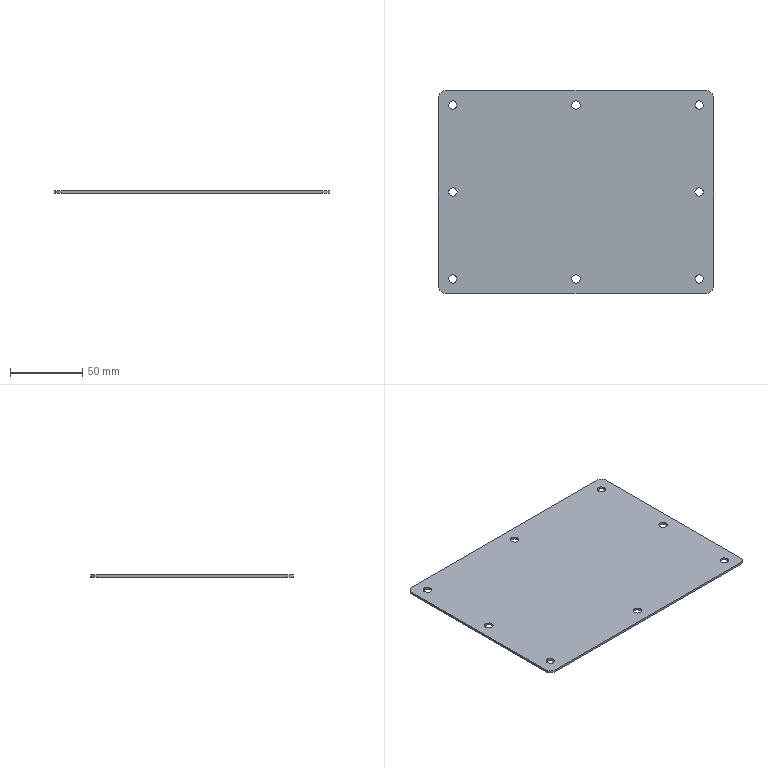Part | SolidWorks | features BreakCorner 1, FlatPattern 1, HoleWzd 1, SMBaseFlange 1, SheetMetal 1 | 1 solid | 26 faces | box 190 x 140 x 1.5 mm | volume 39551 mm3 | cylinder 20 | plane 6 | commonest cylinder face diameters 5.8 x16 10 x4
STEP:
#1=CARTESIAN_POINT('',(-87.9,60.,-1.5));
#2=VERTEX_POINT('',#1);
#3=CARTESIAN_POINT('',(-82.1,60.,-1.5));
#4=VERTEX_POINT('',#3);
#5=CARTESIAN_POINT('',(-85.,60.,-1.5));
#6=DIRECTION('',(0.,0.,1.));
#7=DIRECTION('',(1.,0.,0.));
#8=AXIS2_PLACEMENT_3D('',#5,#6,#7);
#9=CIRCLE('',#8,2.9);
#10=EDGE_CURVE('',#2,#4,#9,.T.);
#11=ORIENTED_EDGE('',*,*,#10,.F.);
#12=CARTESIAN_POINT('',(-87.9,60.,0.));
#13=VERTEX_POINT('',#12);
#14=CARTESIAN_POINT('',(-87.9,60.,0.));
#15=DIRECTION('',(0.,0.,1.));
#16=VECTOR('',#15,1000.);
#17=LINE('',#14,#16);
#18=EDGE_CURVE('',#2,#13,#17,.T.);
#19=ORIENTED_EDGE('',*,*,#18,.T.);
#20=CARTESIAN_POINT('',(-82.1,60.,0.));
#21=VERTEX_POINT('',#20);
#22=CARTESIAN_POINT('',(-85.,60.,0.));
#23=DIRECTION('',(0.,0.,1.));
#24=DIRECTION('',(1.,0.,0.));
#25=AXIS2_PLACEMENT_3D('',#22,#23,#24);
#26=CIRCLE('',#25,2.9);
#27=EDGE_CURVE('',#13,#21,#26,.T.);
#28=ORIENTED_EDGE('',*,*,#27,.T.);
#29=CARTESIAN_POINT('',(-82.1,60.,0.));
#30=DIRECTION('',(0.,0.,1.));
#31=VECTOR('',#30,1000.);
#32=LINE('',#29,#31);
#33=EDGE_CURVE('',#4,#21,#32,.T.);
#34=ORIENTED_EDGE('',*,*,#33,.F.);
#35=EDGE_LOOP('',(#11,#19,#28,#34));
#36=FACE_OUTER_BOUND('',#35,.T.);
#37=CARTESIAN_POINT('',(-85.,60.,0.));
#38=DIRECTION('',(0.,0.,1.));
#39=DIRECTION('',(1.,0.,0.));
#40=AXIS2_PLACEMENT_3D('',#37,#38,#39);
#41=CYLINDRICAL_SURFACE('',#40,2.9);
#42=ADVANCED_FACE('',(#36),#41,.F.);
#43=CARTESIAN_POINT('',(82.1,60.,-1.5));
#44=VERTEX_POINT('',#43);
#45=CARTESIAN_POINT('',(87.9,60.,-1.5));
#46=VERTEX_POINT('',#45);
#47=CARTESIAN_POINT('',(85.,60.,-1.5));
#48=DIRECTION('',(0.,0.,1.));
#49=DIRECTION('',(1.,0.,0.));
#50=AXIS2_PLACEMENT_3D('',#47,#48,#49);
#51=CIRCLE('',#50,2.9);
#52=EDGE_CURVE('',#44,#46,#51,.T.);
#53=ORIENTED_EDGE('',*,*,#52,.F.);
#54=CARTESIAN_POINT('',(82.1,60.,0.));
#55=VERTEX_POINT('',#54);
#56=CARTESIAN_POINT('',(82.1,60.,0.));
#57=DIRECTION('',(0.,0.,1.));
#58=VECTOR('',#57,1000.);
#59=LINE('',#56,#58);
#60=EDGE_CURVE('',#44,#55,#59,.T.);
#61=ORIENTED_EDGE('',*,*,#60,.T.);
#62=CARTESIAN_POINT('',(87.9,60.,0.));
#63=VERTEX_POINT('',#62);
#64=CARTESIAN_POINT('',(85.,60.,0.));
#65=DIRECTION('',(0.,0.,1.));
#66=DIRECTION('',(1.,0.,0.));
#67=AXIS2_PLACEMENT_3D('',#64,#65,#66);
#68=CIRCLE('',#67,2.9);
#69=EDGE_CURVE('',#55,#63,#68,.T.);
#70=ORIENTED_EDGE('',*,*,#69,.T.);
#71=CARTESIAN_POINT('',(87.9,60.,0.));
#72=DIRECTION('',(0.,0.,1.));
#73=VECTOR('',#72,1000.);
#74=LINE('',#71,#73);
#75=EDGE_CURVE('',#46,#63,#74,.T.);
#76=ORIENTED_EDGE('',*,*,#75,.F.);
#77=EDGE_LOOP('',(#53,#61,#70,#76));
#78=FACE_OUTER_BOUND('',#77,.T.);
#79=CARTESIAN_POINT('',(85.,60.,0.));
#80=DIRECTION('',(0.,0.,1.));
#81=DIRECTION('',(1.,0.,0.));
#82=AXIS2_PLACEMENT_3D('',#79,#80,#81);
#83=CYLINDRICAL_SURFACE('',#82,2.9);
#84=ADVANCED_FACE('',(#78),#83,.F.);
#85=CARTESIAN_POINT('',(-87.9,-60.,-1.5));
#86=VERTEX_POINT('',#85);
#87=CARTESIAN_POINT('',(-82.1,-60.,-1.5));
#88=VERTEX_POINT('',#87);
#89=CARTESIAN_POINT('',(-85.,-60.,-1.5));
#90=DIRECTION('',(0.,0.,1.));
#91=DIRECTION('',(1.,0.,0.));
#92=AXIS2_PLACEMENT_3D('',#89,#90,#91);
#93=CIRCLE('',#92,2.9);
#94=EDGE_CURVE('',#86,#88,#93,.T.);
#95=ORIENTED_EDGE('',*,*,#94,.F.);
#96=CARTESIAN_POINT('',(-87.9,-60.,0.));
#97=VERTEX_POINT('',#96);
#98=CARTESIAN_POINT('',(-87.9,-60.,0.));
#99=DIRECTION('',(0.,0.,1.));
#100=VECTOR('',#99,1000.);
#101=LINE('',#98,#100);
#102=EDGE_CURVE('',#86,#97,#101,.T.);
#103=ORIENTED_EDGE('',*,*,#102,.T.);
#104=CARTESIAN_POINT('',(-82.1,-60.,0.));
#105=VERTEX_POINT('',#104);
#106=CARTESIAN_POINT('',(-85.,-60.,0.));
#107=DIRECTION('',(0.,0.,1.));
#108=DIRECTION('',(1.,0.,0.));
#109=AXIS2_PLACEMENT_3D('',#106,#107,#108);
#110=CIRCLE('',#109,2.9);
#111=EDGE_CURVE('',#97,#105,#110,.T.);
#112=ORIENTED_EDGE('',*,*,#111,.T.);
#113=CARTESIAN_POINT('',(-82.1,-60.,0.));
#114=DIRECTION('',(0.,0.,1.));
#115=VECTOR('',#114,1000.);
#116=LINE('',#113,#115);
#117=EDGE_CURVE('',#88,#105,#116,.T.);
#118=ORIENTED_EDGE('',*,*,#117,.F.);
#119=EDGE_LOOP('',(#95,#103,#112,#118));
#120=FACE_OUTER_BOUND('',#119,.T.);
#121=CARTESIAN_POINT('',(-85.,-60.,0.));
#122=DIRECTION('',(0.,0.,1.));
#123=DIRECTION('',(1.,0.,0.));
#124=AXIS2_PLACEMENT_3D('',#121,#122,#123);
#125=CYLINDRICAL_SURFACE('',#124,2.9);
#126=ADVANCED_FACE('',(#120),#125,.F.);
#127=CARTESIAN_POINT('',(82.1,-60.,-1.5));
#128=VERTEX_POINT('',#127);
#129=CARTESIAN_POINT('',(87.9,-60.,-1.5));
#130=VERTEX_POINT('',#129);
#131=CARTESIAN_POINT('',(85.,-60.,-1.5));
#132=DIRECTION('',(0.,0.,1.));
#133=DIRECTION('',(1.,0.,0.));
#134=AXIS2_PLACEMENT_3D('',#131,#132,#133);
#135=CIRCLE('',#134,2.9);
#136=EDGE_CURVE('',#128,#130,#135,.T.);
#137=ORIENTED_EDGE('',*,*,#136,.F.);
#138=CARTESIAN_POINT('',(82.1,-60.,0.));
#139=VERTEX_POINT('',#138);
#140=CARTESIAN_POINT('',(82.1,-60.,0.));
#141=DIRECTION('',(0.,0.,1.));
#142=VECTOR('',#141,1000.);
#143=LINE('',#140,#142);
#144=EDGE_CURVE('',#128,#139,#143,.T.);
#145=ORIENTED_EDGE('',*,*,#144,.T.);
#146=CARTESIAN_POINT('',(87.9,-60.,0.));
#147=VERTEX_POINT('',#146);
#148=CARTESIAN_POINT('',(85.,-60.,0.));
#149=DIRECTION('',(0.,0.,1.));
#150=DIRECTION('',(1.,0.,0.));
#151=AXIS2_PLACEMENT_3D('',#148,#149,#150);
#152=CIRCLE('',#151,2.9);
#153=EDGE_CURVE('',#139,#147,#152,.T.);
#154=ORIENTED_EDGE('',*,*,#153,.T.);
#155=CARTESIAN_POINT('',(87.9,-60.,0.));
#156=DIRECTION('',(0.,0.,1.));
#157=VECTOR('',#156,1000.);
#158=LINE('',#155,#157);
#159=EDGE_CURVE('',#130,#147,#158,.T.);
#160=ORIENTED_EDGE('',*,*,#159,.F.);
#161=EDGE_LOOP('',(#137,#145,#154,#160));
#162=FACE_OUTER_BOUND('',#161,.T.);
#163=CARTESIAN_POINT('',(85.,-60.,0.));
#164=DIRECTION('',(0.,0.,1.));
#165=DIRECTION('',(1.,0.,0.));
#166=AXIS2_PLACEMENT_3D('',#163,#164,#165);
#167=CYLINDRICAL_SURFACE('',#166,2.9);
#168=ADVANCED_FACE('',(#162),#167,.F.);
#169=CARTESIAN_POINT('',(-87.9,0.,-1.5));
#170=VERTEX_POINT('',#169);
#171=CARTESIAN_POINT('',(-82.1,0.,-1.5));
#172=VERTEX_POINT('',#171);
#173=CARTESIAN_POINT('',(-85.,0.,-1.5));
#174=DIRECTION('',(0.,0.,1.));
#175=DIRECTION('',(1.,0.,0.));
#176=AXIS2_PLACEMENT_3D('',#173,#174,#175);
#177=CIRCLE('',#176,2.9);
#178=EDGE_CURVE('',#170,#172,#177,.T.);
#179=ORIENTED_EDGE('',*,*,#178,.F.);
#180=CARTESIAN_POINT('',(-87.9,0.,0.));
#181=VERTEX_POINT('',#180);
#182=CARTESIAN_POINT('',(-87.9,0.,0.));
#183=DIRECTION('',(0.,0.,1.));
#184=VECTOR('',#183,1000.);
#185=LINE('',#182,#184);
#186=EDGE_CURVE('',#170,#181,#185,.T.);
#187=ORIENTED_EDGE('',*,*,#186,.T.);
#188=CARTESIAN_POINT('',(-82.1,0.,0.));
#189=VERTEX_POINT('',#188);
#190=CARTESIAN_POINT('',(-85.,0.,0.));
#191=DIRECTION('',(0.,0.,1.));
#192=DIRECTION('',(1.,0.,0.));
#193=AXIS2_PLACEMENT_3D('',#190,#191,#192);
#194=CIRCLE('',#193,2.9);
#195=EDGE_CURVE('',#181,#189,#194,.T.);
#196=ORIENTED_EDGE('',*,*,#195,.T.);
#197=CARTESIAN_POINT('',(-82.1,0.,0.));
#198=DIRECTION('',(0.,0.,1.));
#199=VECTOR('',#198,1000.);
#200=LINE('',#197,#199);
#201=EDGE_CURVE('',#172,#189,#200,.T.);
#202=ORIENTED_EDGE('',*,*,#201,.F.);
#203=EDGE_LOOP('',(#179,#187,#196,#202));
#204=FACE_OUTER_BOUND('',#203,.T.);
#205=CARTESIAN_POINT('',(-85.,0.,0.));
#206=DIRECTION('',(0.,0.,1.));
#207=DIRECTION('',(1.,0.,0.));
#208=AXIS2_PLACEMENT_3D('',#205,#206,#207);
#209=CYLINDRICAL_SURFACE('',#208,2.9);
#210=ADVANCED_FACE('',(#204),#209,.F.);
#211=CARTESIAN_POINT('',(82.1,0.,-1.5));
#212=VERTEX_POINT('',#211);
#213=CARTESIAN_POINT('',(87.9,0.,-1.5));
#214=VERTEX_POINT('',#213);
#215=CARTESIAN_POINT('',(85.,0.,-1.5));
#216=DIRECTION('',(0.,0.,1.));
#217=DIRECTION('',(1.,0.,0.));
#218=AXIS2_PLACEMENT_3D('',#215,#216,#217);
#219=CIRCLE('',#218,2.9);
#220=EDGE_CURVE('',#212,#214,#219,.T.);
#221=ORIENTED_EDGE('',*,*,#220,.F.);
#222=CARTESIAN_POINT('',(82.1,0.,0.));
#223=VERTEX_POINT('',#222);
#224=CARTESIAN_POINT('',(82.1,0.,0.));
#225=DIRECTION('',(0.,0.,1.));
#226=VECTOR('',#225,1000.);
#227=LINE('',#224,#226);
#228=EDGE_CURVE('',#212,#223,#227,.T.);
#229=ORIENTED_EDGE('',*,*,#228,.T.);
#230=CARTESIAN_POINT('',(87.9,0.,0.));
#231=VERTEX_POINT('',#230);
#232=CARTESIAN_POINT('',(85.,0.,0.));
#233=DIRECTION('',(0.,0.,1.));
#234=DIRECTION('',(1.,0.,0.));
#235=AXIS2_PLACEMENT_3D('',#232,#233,#234);
#236=CIRCLE('',#235,2.9);
#237=EDGE_CURVE('',#223,#231,#236,.T.);
#238=ORIENTED_EDGE('',*,*,#237,.T.);
#239=CARTESIAN_POINT('',(87.9,0.,0.));
#240=DIRECTION('',(0.,0.,1.));
#241=VECTOR('',#240,1000.);
#242=LINE('',#239,#241);
#243=EDGE_CURVE('',#214,#231,#242,.T.);
#244=ORIENTED_EDGE('',*,*,#243,.F.);
#245=EDGE_LOOP('',(#221,#229,#238,#244));
#246=FACE_OUTER_BOUND('',#245,.T.);
#247=CARTESIAN_POINT('',(85.,0.,0.));
#248=DIRECTION('',(0.,0.,1.));
#249=DIRECTION('',(1.,0.,0.));
#250=AXIS2_PLACEMENT_3D('',#247,#248,#249);
#251=CYLINDRICAL_SURFACE('',#250,2.9);
#252=ADVANCED_FACE('',(#246),#251,.F.);
#253=CARTESIAN_POINT('',(-2.9,-60.,-1.5));
#254=VERTEX_POINT('',#253);
#255=CARTESIAN_POINT('',(2.9,-60.,-1.5));
#256=VERTEX_POINT('',#255);
#257=CARTESIAN_POINT('',(0.,-60.,-1.5));
#258=DIRECTION('',(0.,0.,1.));
#259=DIRECTION('',(1.,0.,0.));
#260=AXIS2_PLACEMENT_3D('',#257,#258,#259);
#261=CIRCLE('',#260,2.9);
#262=EDGE_CURVE('',#254,#256,#261,.T.);
#263=ORIENTED_EDGE('',*,*,#262,.F.);
#264=CARTESIAN_POINT('',(-2.9,-60.,0.));
#265=VERTEX_POINT('',#264);
#266=CARTESIAN_POINT('',(-2.9,-60.,0.));
#267=DIRECTION('',(0.,0.,1.));
#268=VECTOR('',#267,1000.);
#269=LINE('',#266,#268);
#270=EDGE_CURVE('',#254,#265,#269,.T.);
#271=ORIENTED_EDGE('',*,*,#270,.T.);
#272=CARTESIAN_POINT('',(2.9,-60.,0.));
#273=VERTEX_POINT('',#272);
#274=CARTESIAN_POINT('',(0.,-60.,0.));
#275=DIRECTION('',(0.,0.,1.));
#276=DIRECTION('',(1.,0.,0.));
#277=AXIS2_PLACEMENT_3D('',#274,#275,#276);
#278=CIRCLE('',#277,2.9);
#279=EDGE_CURVE('',#265,#273,#278,.T.);
#280=ORIENTED_EDGE('',*,*,#279,.T.);
#281=CARTESIAN_POINT('',(2.9,-60.,0.));
#282=DIRECTION('',(0.,0.,1.));
#283=VECTOR('',#282,1000.);
#284=LINE('',#281,#283);
#285=EDGE_CURVE('',#256,#273,#284,.T.);
#286=ORIENTED_EDGE('',*,*,#285,.F.);
#287=EDGE_LOOP('',(#263,#271,#280,#286));
#288=FACE_OUTER_BOUND('',#287,.T.);
#289=CARTESIAN_POINT('',(0.,-60.,0.));
#290=DIRECTION('',(0.,0.,1.));
#291=DIRECTION('',(1.,0.,0.));
#292=AXIS2_PLACEMENT_3D('',#289,#290,#291);
#293=CYLINDRICAL_SURFACE('',#292,2.9);
#294=ADVANCED_FACE('',(#288),#293,.F.);
#295=CARTESIAN_POINT('',(-2.9,60.,-1.5));
#296=VERTEX_POINT('',#295);
#297=CARTESIAN_POINT('',(2.9,60.,-1.5));
#298=VERTEX_POINT('',#297);
#299=CARTESIAN_POINT('',(0.,60.,-1.5));
#300=DIRECTION('',(0.,0.,1.));
#301=DIRECTION('',(1.,0.,0.));
#302=AXIS2_PLACEMENT_3D('',#299,#300,#301);
#303=CIRCLE('',#302,2.9);
#304=EDGE_CURVE('',#296,#298,#303,.T.);
#305=ORIENTED_EDGE('',*,*,#304,.F.);
#306=CARTESIAN_POINT('',(-2.9,60.,0.));
#307=VERTEX_POINT('',#306);
#308=CARTESIAN_POINT('',(-2.9,60.,0.));
#309=DIRECTION('',(0.,0.,1.));
#310=VECTOR('',#309,1000.);
#311=LINE('',#308,#310);
#312=EDGE_CURVE('',#296,#307,#311,.T.);
#313=ORIENTED_EDGE('',*,*,#312,.T.);
#314=CARTESIAN_POINT('',(2.9,60.,0.));
#315=VERTEX_POINT('',#314);
#316=CARTESIAN_POINT('',(0.,60.,0.));
#317=DIRECTION('',(0.,0.,1.));
#318=DIRECTION('',(1.,0.,0.));
#319=AXIS2_PLACEMENT_3D('',#316,#317,#318);
#320=CIRCLE('',#319,2.9);
#321=EDGE_CURVE('',#307,#315,#320,.T.);
#322=ORIENTED_EDGE('',*,*,#321,.T.);
#323=CARTESIAN_POINT('',(2.9,60.,0.));
#324=DIRECTION('',(0.,0.,1.));
#325=VECTOR('',#324,1000.);
#326=LINE('',#323,#325);
#327=EDGE_CURVE('',#298,#315,#326,.T.);
#328=ORIENTED_EDGE('',*,*,#327,.F.);
#329=EDGE_LOOP('',(#305,#313,#322,#328));
#330=FACE_OUTER_BOUND('',#329,.T.);
#331=CARTESIAN_POINT('',(0.,60.,0.));
#332=DIRECTION('',(0.,0.,1.));
#333=DIRECTION('',(1.,0.,0.));
#334=AXIS2_PLACEMENT_3D('',#331,#332,#333);
#335=CYLINDRICAL_SURFACE('',#334,2.9);
#336=ADVANCED_FACE('',(#330),#335,.F.);
#337=CARTESIAN_POINT('',(-85.,60.,0.));
#338=DIRECTION('',(0.,0.,1.));
#339=DIRECTION('',(1.,0.,0.));
#340=AXIS2_PLACEMENT_3D('',#337,#338,#339);
#341=CIRCLE('',#340,2.9);
#342=EDGE_CURVE('',#21,#13,#341,.T.);
#343=ORIENTED_EDGE('',*,*,#342,.F.);
#344=ORIENTED_EDGE('',*,*,#27,.F.);
#345=EDGE_LOOP('',(#343,#344));
#346=FACE_BOUND('',#345,.T.);
#347=CARTESIAN_POINT('',(85.,60.,0.));
#348=DIRECTION('',(0.,0.,1.));
#349=DIRECTION('',(1.,0.,0.));
#350=AXIS2_PLACEMENT_3D('',#347,#348,#349);
#351=CIRCLE('',#350,2.9);
#352=EDGE_CURVE('',#63,#55,#351,.T.);
#353=ORIENTED_EDGE('',*,*,#352,.F.);
#354=ORIENTED_EDGE('',*,*,#69,.F.);
#355=EDGE_LOOP('',(#353,#354));
#356=FACE_BOUND('',#355,.T.);
#357=CARTESIAN_POINT('',(-85.,-60.,0.));
#358=DIRECTION('',(0.,0.,1.));
#359=DIRECTION('',(1.,0.,0.));
#360=AXIS2_PLACEMENT_3D('',#357,#358,#359);
#361=CIRCLE('',#360,2.9);
#362=EDGE_CURVE('',#105,#97,#361,.T.);
#363=ORIENTED_EDGE('',*,*,#362,.F.);
#364=ORIENTED_EDGE('',*,*,#111,.F.);
#365=EDGE_LOOP('',(#363,#364));
#366=FACE_BOUND('',#365,.T.);
#367=CARTESIAN_POINT('',(85.,-60.,0.));
#368=DIRECTION('',(0.,0.,1.));
#369=DIRECTION('',(1.,0.,0.));
#370=AXIS2_PLACEMENT_3D('',#367,#368,#369);
#371=CIRCLE('',#370,2.9);
#372=EDGE_CURVE('',#147,#139,#371,.T.);
#373=ORIENTED_EDGE('',*,*,#372,.F.);
#374=ORIENTED_EDGE('',*,*,#153,.F.);
#375=EDGE_LOOP('',(#373,#374));
#376=FACE_BOUND('',#375,.T.);
#377=CARTESIAN_POINT('',(-85.,0.,0.));
#378=DIRECTION('',(0.,0.,1.));
#379=DIRECTION('',(1.,0.,0.));
#380=AXIS2_PLACEMENT_3D('',#377,#378,#379);
#381=CIRCLE('',#380,2.9);
#382=EDGE_CURVE('',#189,#181,#381,.T.);
#383=ORIENTED_EDGE('',*,*,#382,.F.);
#384=ORIENTED_EDGE('',*,*,#195,.F.);
#385=EDGE_LOOP('',(#383,#384));
#386=FACE_BOUND('',#385,.T.);
#387=CARTESIAN_POINT('',(0.,-60.,0.));
#388=DIRECTION('',(0.,0.,1.));
#389=DIRECTION('',(1.,0.,0.));
#390=AXIS2_PLACEMENT_3D('',#387,#388,#389);
#391=CIRCLE('',#390,2.9);
#392=EDGE_CURVE('',#273,#265,#391,.T.);
#393=ORIENTED_EDGE('',*,*,#392,.F.);
#394=ORIENTED_EDGE('',*,*,#279,.F.);
#395=EDGE_LOOP('',(#393,#394));
#396=FACE_BOUND('',#395,.T.);
#397=CARTESIAN_POINT('',(0.,60.,0.));
#398=DIRECTION('',(0.,0.,1.));
#399=DIRECTION('',(1.,0.,0.));
#400=AXIS2_PLACEMENT_3D('',#397,#398,#399);
#401=CIRCLE('',#400,2.9);
#402=EDGE_CURVE('',#315,#307,#401,.T.);
#403=ORIENTED_EDGE('',*,*,#402,.F.);
#404=ORIENTED_EDGE('',*,*,#321,.F.);
#405=EDGE_LOOP('',(#403,#404));
#406=FACE_BOUND('',#405,.T.);
#407=CARTESIAN_POINT('',(-90.,-70.,0.));
#408=VERTEX_POINT('',#407);
#409=CARTESIAN_POINT('',(90.,-70.,0.));
#410=VERTEX_POINT('',#409);
#411=CARTESIAN_POINT('',(-95.,-70.,0.));
#412=DIRECTION('',(1.,0.,0.));
#413=VECTOR('',#412,1000.);
#414=LINE('',#411,#413);
#415=EDGE_CURVE('',#408,#410,#414,.T.);
#416=ORIENTED_EDGE('',*,*,#415,.T.);
#417=CARTESIAN_POINT('',(95.,-65.,0.));
#418=VERTEX_POINT('',#417);
#419=CARTESIAN_POINT('',(90.,-65.,0.));
#420=DIRECTION('',(0.,0.,1.));
#421=DIRECTION('',(-1.,0.,0.));
#422=AXIS2_PLACEMENT_3D('',#419,#420,#421);
#423=CIRCLE('',#422,5.);
#424=EDGE_CURVE('',#410,#418,#423,.T.);
#425=ORIENTED_EDGE('',*,*,#424,.T.);
#426=CARTESIAN_POINT('',(95.,65.,0.));
#427=VERTEX_POINT('',#426);
#428=CARTESIAN_POINT('',(95.,-70.,0.));
#429=DIRECTION('',(0.,1.,0.));
#430=VECTOR('',#429,1000.);
#431=LINE('',#428,#430);
#432=EDGE_CURVE('',#418,#427,#431,.T.);
#433=ORIENTED_EDGE('',*,*,#432,.T.);
#434=CARTESIAN_POINT('',(90.,70.,0.));
#435=VERTEX_POINT('',#434);
#436=CARTESIAN_POINT('',(90.,65.,0.));
#437=DIRECTION('',(0.,0.,1.));
#438=DIRECTION('',(-1.,0.,0.));
#439=AXIS2_PLACEMENT_3D('',#436,#437,#438);
#440=CIRCLE('',#439,5.);
#441=EDGE_CURVE('',#427,#435,#440,.T.);
#442=ORIENTED_EDGE('',*,*,#441,.T.);
#443=CARTESIAN_POINT('',(-90.,70.,0.));
#444=VERTEX_POINT('',#443);
#445=CARTESIAN_POINT('',(-95.,70.,0.));
#446=DIRECTION('',(-1.,0.,0.));
#447=VECTOR('',#446,1000.);
#448=LINE('',#445,#447);
#449=EDGE_CURVE('',#435,#444,#448,.T.);
#450=ORIENTED_EDGE('',*,*,#449,.T.);
#451=CARTESIAN_POINT('',(-95.,65.,0.));
#452=VERTEX_POINT('',#451);
#453=CARTESIAN_POINT('',(-90.,65.,0.));
#454=DIRECTION('',(0.,0.,1.));
#455=DIRECTION('',(-1.,0.,0.));
#456=AXIS2_PLACEMENT_3D('',#453,#454,#455);
#457=CIRCLE('',#456,5.);
#458=EDGE_CURVE('',#444,#452,#457,.T.);
#459=ORIENTED_EDGE('',*,*,#458,.T.);
#460=CARTESIAN_POINT('',(-95.,-65.,0.));
#461=VERTEX_POINT('',#460);
#462=CARTESIAN_POINT('',(-95.,-70.,0.));
#463=DIRECTION('',(0.,-1.,0.));
#464=VECTOR('',#463,1000.);
#465=LINE('',#462,#464);
#466=EDGE_CURVE('',#452,#461,#465,.T.);
#467=ORIENTED_EDGE('',*,*,#466,.T.);
#468=CARTESIAN_POINT('',(-90.,-65.,0.));
#469=DIRECTION('',(0.,0.,1.));
#470=DIRECTION('',(-1.,0.,0.));
#471=AXIS2_PLACEMENT_3D('',#468,#469,#470);
#472=CIRCLE('',#471,5.);
#473=EDGE_CURVE('',#461,#408,#472,.T.);
#474=ORIENTED_EDGE('',*,*,#473,.T.);
#475=EDGE_LOOP('',(#416,#425,#433,#442,#450,#459,#467,#474));
#476=FACE_OUTER_BOUND('',#475,.T.);
#477=CARTESIAN_POINT('',(85.,0.,0.));
#478=DIRECTION('',(0.,0.,1.));
#479=DIRECTION('',(1.,0.,0.));
#480=AXIS2_PLACEMENT_3D('',#477,#478,#479);
#481=CIRCLE('',#480,2.9);
#482=EDGE_CURVE('',#231,#223,#481,.T.);
#483=ORIENTED_EDGE('',*,*,#482,.F.);
#484=ORIENTED_EDGE('',*,*,#237,.F.);
#485=EDGE_LOOP('',(#483,#484));
#486=FACE_BOUND('',#485,.T.);
#487=CARTESIAN_POINT('',(0.,0.,0.));
#488=DIRECTION('',(0.,0.,-1.));
#489=DIRECTION('',(-1.,0.,0.));
#490=AXIS2_PLACEMENT_3D('',#487,#488,#489);
#491=PLANE('',#490);
#492=ADVANCED_FACE('',(#346,#356,#366,#376,#386,#396,#406,#476,#486),#491,.F.);
#493=ORIENTED_EDGE('',*,*,#432,.F.);
#494=CARTESIAN_POINT('',(95.,-65.,-1.5));
#495=VERTEX_POINT('',#494);
#496=CARTESIAN_POINT('',(95.,-65.,-1.5));
#497=DIRECTION('',(0.,0.,-1.));
#498=VECTOR('',#497,1000.);
#499=LINE('',#496,#498);
#500=EDGE_CURVE('',#418,#495,#499,.T.);
#501=ORIENTED_EDGE('',*,*,#500,.T.);
#502=CARTESIAN_POINT('',(95.,65.,-1.5));
#503=VERTEX_POINT('',#502);
#504=CARTESIAN_POINT('',(95.,-70.,-1.5));
#505=DIRECTION('',(0.,1.,0.));
#506=VECTOR('',#505,1000.);
#507=LINE('',#504,#506);
#508=EDGE_CURVE('',#495,#503,#507,.T.);
#509=ORIENTED_EDGE('',*,*,#508,.T.);
#510=CARTESIAN_POINT('',(95.,65.,-1.5));
#511=DIRECTION('',(0.,0.,1.));
#512=VECTOR('',#511,1000.);
#513=LINE('',#510,#512);
#514=EDGE_CURVE('',#503,#427,#513,.T.);
#515=ORIENTED_EDGE('',*,*,#514,.T.);
#516=EDGE_LOOP('',(#493,#501,#509,#515));
#517=FACE_OUTER_BOUND('',#516,.T.);
#518=CARTESIAN_POINT('',(95.,-70.,-1.5));
#519=DIRECTION('',(1.,0.,0.));
#520=DIRECTION('',(0.,0.,-1.));
#521=AXIS2_PLACEMENT_3D('',#518,#519,#520);
#522=PLANE('',#521);
#523=ADVANCED_FACE('',(#517),#522,.T.);
#524=CARTESIAN_POINT('',(-90.,-70.,-1.5));
#525=VERTEX_POINT('',#524);
#526=CARTESIAN_POINT('',(90.,-70.,-1.5));
#527=VERTEX_POINT('',#526);
#528=CARTESIAN_POINT('',(-95.,-70.,-1.5));
#529=DIRECTION('',(1.,0.,0.));
#530=VECTOR('',#529,1000.);
#531=LINE('',#528,#530);
#532=EDGE_CURVE('',#525,#527,#531,.T.);
#533=ORIENTED_EDGE('',*,*,#532,.T.);
#534=CARTESIAN_POINT('',(90.,-70.,-1.5));
#535=DIRECTION('',(0.,0.,1.));
#536=VECTOR('',#535,1000.);
#537=LINE('',#534,#536);
#538=EDGE_CURVE('',#527,#410,#537,.T.);
#539=ORIENTED_EDGE('',*,*,#538,.T.);
#540=ORIENTED_EDGE('',*,*,#415,.F.);
#541=CARTESIAN_POINT('',(-90.,-70.,-1.5));
#542=DIRECTION('',(0.,0.,-1.));
#543=VECTOR('',#542,1000.);
#544=LINE('',#541,#543);
#545=EDGE_CURVE('',#408,#525,#544,.T.);
#546=ORIENTED_EDGE('',*,*,#545,.T.);
#547=EDGE_LOOP('',(#533,#539,#540,#546));
#548=FACE_OUTER_BOUND('',#547,.T.);
#549=CARTESIAN_POINT('',(-95.,-70.,-1.5));
#550=DIRECTION('',(0.,-1.,0.));
#551=DIRECTION('',(0.,0.,-1.));
#552=AXIS2_PLACEMENT_3D('',#549,#550,#551);
#553=PLANE('',#552);
#554=ADVANCED_FACE('',(#548),#553,.T.);
#555=CARTESIAN_POINT('',(-95.,65.,-1.5));
#556=VERTEX_POINT('',#555);
#557=CARTESIAN_POINT('',(-95.,-65.,-1.5));
#558=VERTEX_POINT('',#557);
#559=CARTESIAN_POINT('',(-95.,-70.,-1.5));
#560=DIRECTION('',(0.,-1.,0.));
#561=VECTOR('',#560,1000.);
#562=LINE('',#559,#561);
#563=EDGE_CURVE('',#556,#558,#562,.T.);
#564=ORIENTED_EDGE('',*,*,#563,.T.);
#565=CARTESIAN_POINT('',(-95.,-65.,-1.5));
#566=DIRECTION('',(0.,0.,1.));
#567=VECTOR('',#566,1000.);
#568=LINE('',#565,#567);
#569=EDGE_CURVE('',#558,#461,#568,.T.);
#570=ORIENTED_EDGE('',*,*,#569,.T.);
#571=ORIENTED_EDGE('',*,*,#466,.F.);
#572=CARTESIAN_POINT('',(-95.,65.,-1.5));
#573=DIRECTION('',(0.,0.,-1.));
#574=VECTOR('',#573,1000.);
#575=LINE('',#572,#574);
#576=EDGE_CURVE('',#452,#556,#575,.T.);
#577=ORIENTED_EDGE('',*,*,#576,.T.);
#578=EDGE_LOOP('',(#564,#570,#571,#577));
#579=FACE_OUTER_BOUND('',#578,.T.);
#580=CARTESIAN_POINT('',(-95.,-70.,-1.5));
#581=DIRECTION('',(-1.,0.,0.));
#582=DIRECTION('',(0.,0.,1.));
#583=AXIS2_PLACEMENT_3D('',#580,#581,#582);
#584=PLANE('',#583);
#585=ADVANCED_FACE('',(#579),#584,.T.);
#586=CARTESIAN_POINT('',(90.,70.,-1.5));
#587=VERTEX_POINT('',#586);
#588=CARTESIAN_POINT('',(-90.,70.,-1.5));
#589=VERTEX_POINT('',#588);
#590=CARTESIAN_POINT('',(-95.,70.,-1.5));
#591=DIRECTION('',(-1.,0.,0.));
#592=VECTOR('',#591,1000.);
#593=LINE('',#590,#592);
#594=EDGE_CURVE('',#587,#589,#593,.T.);
#595=ORIENTED_EDGE('',*,*,#594,.T.);
#596=CARTESIAN_POINT('',(-90.,70.,-1.5));
#597=DIRECTION('',(0.,0.,1.));
#598=VECTOR('',#597,1000.);
#599=LINE('',#596,#598);
#600=EDGE_CURVE('',#589,#444,#599,.T.);
#601=ORIENTED_EDGE('',*,*,#600,.T.);
#602=ORIENTED_EDGE('',*,*,#449,.F.);
#603=CARTESIAN_POINT('',(90.,70.,-1.5));
#604=DIRECTION('',(0.,0.,-1.));
#605=VECTOR('',#604,1000.);
#606=LINE('',#603,#605);
#607=EDGE_CURVE('',#435,#587,#606,.T.);
#608=ORIENTED_EDGE('',*,*,#607,.T.);
#609=EDGE_LOOP('',(#595,#601,#602,#608));
#610=FACE_OUTER_BOUND('',#609,.T.);
#611=CARTESIAN_POINT('',(-95.,70.,-1.5));
#612=DIRECTION('',(0.,1.,0.));
#613=DIRECTION('',(0.,0.,1.));
#614=AXIS2_PLACEMENT_3D('',#611,#612,#613);
#615=PLANE('',#614);
#616=ADVANCED_FACE('',(#610),#615,.T.);
#617=CARTESIAN_POINT('',(-85.,60.,-1.5));
#618=DIRECTION('',(0.,0.,1.));
#619=DIRECTION('',(1.,0.,0.));
#620=AXIS2_PLACEMENT_3D('',#617,#618,#619);
#621=CIRCLE('',#620,2.9);
#622=EDGE_CURVE('',#4,#2,#621,.T.);
#623=ORIENTED_EDGE('',*,*,#622,.T.);
#624=ORIENTED_EDGE('',*,*,#10,.T.);
#625=EDGE_LOOP('',(#623,#624));
#626=FACE_BOUND('',#625,.T.);
#627=CARTESIAN_POINT('',(85.,60.,-1.5));
#628=DIRECTION('',(0.,0.,1.));
#629=DIRECTION('',(1.,0.,0.));
#630=AXIS2_PLACEMENT_3D('',#627,#628,#629);
#631=CIRCLE('',#630,2.9);
#632=EDGE_CURVE('',#46,#44,#631,.T.);
#633=ORIENTED_EDGE('',*,*,#632,.T.);
#634=ORIENTED_EDGE('',*,*,#52,.T.);
#635=EDGE_LOOP('',(#633,#634));
#636=FACE_BOUND('',#635,.T.);
#637=CARTESIAN_POINT('',(-85.,-60.,-1.5));
#638=DIRECTION('',(0.,0.,1.));
#639=DIRECTION('',(1.,0.,0.));
#640=AXIS2_PLACEMENT_3D('',#637,#638,#639);
#641=CIRCLE('',#640,2.9);
#642=EDGE_CURVE('',#88,#86,#641,.T.);
#643=ORIENTED_EDGE('',*,*,#642,.T.);
#644=ORIENTED_EDGE('',*,*,#94,.T.);
#645=EDGE_LOOP('',(#643,#644));
#646=FACE_BOUND('',#645,.T.);
#647=CARTESIAN_POINT('',(85.,-60.,-1.5));
#648=DIRECTION('',(0.,0.,1.));
#649=DIRECTION('',(1.,0.,0.));
#650=AXIS2_PLACEMENT_3D('',#647,#648,#649);
#651=CIRCLE('',#650,2.9);
#652=EDGE_CURVE('',#130,#128,#651,.T.);
#653=ORIENTED_EDGE('',*,*,#652,.T.);
#654=ORIENTED_EDGE('',*,*,#136,.T.);
#655=EDGE_LOOP('',(#653,#654));
#656=FACE_BOUND('',#655,.T.);
#657=CARTESIAN_POINT('',(-85.,0.,-1.5));
#658=DIRECTION('',(0.,0.,1.));
#659=DIRECTION('',(1.,0.,0.));
#660=AXIS2_PLACEMENT_3D('',#657,#658,#659);
#661=CIRCLE('',#660,2.9);
#662=EDGE_CURVE('',#172,#170,#661,.T.);
#663=ORIENTED_EDGE('',*,*,#662,.T.);
#664=ORIENTED_EDGE('',*,*,#178,.T.);
#665=EDGE_LOOP('',(#663,#664));
#666=FACE_BOUND('',#665,.T.);
#667=CARTESIAN_POINT('',(85.,0.,-1.5));
#668=DIRECTION('',(0.,0.,1.));
#669=DIRECTION('',(1.,0.,0.));
#670=AXIS2_PLACEMENT_3D('',#667,#668,#669);
#671=CIRCLE('',#670,2.9);
#672=EDGE_CURVE('',#214,#212,#671,.T.);
#673=ORIENTED_EDGE('',*,*,#672,.T.);
#674=ORIENTED_EDGE('',*,*,#220,.T.);
#675=EDGE_LOOP('',(#673,#674));
#676=FACE_BOUND('',#675,.T.);
#677=CARTESIAN_POINT('',(0.,-60.,-1.5));
#678=DIRECTION('',(0.,0.,1.));
#679=DIRECTION('',(1.,0.,0.));
#680=AXIS2_PLACEMENT_3D('',#677,#678,#679);
#681=CIRCLE('',#680,2.9);
#682=EDGE_CURVE('',#256,#254,#681,.T.);
#683=ORIENTED_EDGE('',*,*,#682,.T.);
#684=ORIENTED_EDGE('',*,*,#262,.T.);
#685=EDGE_LOOP('',(#683,#684));
#686=FACE_BOUND('',#685,.T.);
#687=CARTESIAN_POINT('',(0.,60.,-1.5));
#688=DIRECTION('',(0.,0.,1.));
#689=DIRECTION('',(1.,0.,0.));
#690=AXIS2_PLACEMENT_3D('',#687,#688,#689);
#691=CIRCLE('',#690,2.9);
#692=EDGE_CURVE('',#298,#296,#691,.T.);
#693=ORIENTED_EDGE('',*,*,#692,.T.);
#694=ORIENTED_EDGE('',*,*,#304,.T.);
#695=EDGE_LOOP('',(#693,#694));
#696=FACE_BOUND('',#695,.T.);
#697=ORIENTED_EDGE('',*,*,#508,.F.);
#698=CARTESIAN_POINT('',(90.,-65.,-1.5));
#699=DIRECTION('',(0.,0.,-1.));
#700=DIRECTION('',(-1.,0.,0.));
#701=AXIS2_PLACEMENT_3D('',#698,#699,#700);
#702=CIRCLE('',#701,5.);
#703=EDGE_CURVE('',#495,#527,#702,.T.);
#704=ORIENTED_EDGE('',*,*,#703,.T.);
#705=ORIENTED_EDGE('',*,*,#532,.F.);
#706=CARTESIAN_POINT('',(-90.,-65.,-1.5));
#707=DIRECTION('',(0.,0.,-1.));
#708=DIRECTION('',(-1.,0.,0.));
#709=AXIS2_PLACEMENT_3D('',#706,#707,#708);
#710=CIRCLE('',#709,5.);
#711=EDGE_CURVE('',#525,#558,#710,.T.);
#712=ORIENTED_EDGE('',*,*,#711,.T.);
#713=ORIENTED_EDGE('',*,*,#563,.F.);
#714=CARTESIAN_POINT('',(-90.,65.,-1.5));
#715=DIRECTION('',(0.,0.,-1.));
#716=DIRECTION('',(-1.,0.,0.));
#717=AXIS2_PLACEMENT_3D('',#714,#715,#716);
#718=CIRCLE('',#717,5.);
#719=EDGE_CURVE('',#556,#589,#718,.T.);
#720=ORIENTED_EDGE('',*,*,#719,.T.);
#721=ORIENTED_EDGE('',*,*,#594,.F.);
#722=CARTESIAN_POINT('',(90.,65.,-1.5));
#723=DIRECTION('',(0.,0.,-1.));
#724=DIRECTION('',(-1.,0.,0.));
#725=AXIS2_PLACEMENT_3D('',#722,#723,#724);
#726=CIRCLE('',#725,5.);
#727=EDGE_CURVE('',#587,#503,#726,.T.);
#728=ORIENTED_EDGE('',*,*,#727,.T.);
#729=EDGE_LOOP('',(#697,#704,#705,#712,#713,#720,#721,#728));
#730=FACE_OUTER_BOUND('',#729,.T.);
#731=CARTESIAN_POINT('',(0.,0.,-1.5));
#732=DIRECTION('',(0.,0.,-1.));
#733=DIRECTION('',(-1.,0.,0.));
#734=AXIS2_PLACEMENT_3D('',#731,#732,#733);
#735=PLANE('',#734);
#736=ADVANCED_FACE('',(#626,#636,#646,#656,#666,#676,#686,#696,#730),#735,.T.);
#737=ORIENTED_EDGE('',*,*,#312,.F.);
#738=ORIENTED_EDGE('',*,*,#692,.F.);
#739=ORIENTED_EDGE('',*,*,#327,.T.);
#740=ORIENTED_EDGE('',*,*,#402,.T.);
#741=EDGE_LOOP('',(#737,#738,#739,#740));
#742=FACE_OUTER_BOUND('',#741,.T.);
#743=CARTESIAN_POINT('',(0.,60.,0.));
#744=DIRECTION('',(0.,0.,1.));
#745=DIRECTION('',(1.,0.,0.));
#746=AXIS2_PLACEMENT_3D('',#743,#744,#745);
#747=CYLINDRICAL_SURFACE('',#746,2.9);
#748=ADVANCED_FACE('',(#742),#747,.F.);
#749=ORIENTED_EDGE('',*,*,#270,.F.);
#750=ORIENTED_EDGE('',*,*,#682,.F.);
#751=ORIENTED_EDGE('',*,*,#285,.T.);
#752=ORIENTED_EDGE('',*,*,#392,.T.);
#753=EDGE_LOOP('',(#749,#750,#751,#752));
#754=FACE_OUTER_BOUND('',#753,.T.);
#755=CARTESIAN_POINT('',(0.,-60.,0.));
#756=DIRECTION('',(0.,0.,1.));
#757=DIRECTION('',(1.,0.,0.));
#758=AXIS2_PLACEMENT_3D('',#755,#756,#757);
#759=CYLINDRICAL_SURFACE('',#758,2.9);
#760=ADVANCED_FACE('',(#754),#759,.F.);
#761=ORIENTED_EDGE('',*,*,#228,.F.);
#762=ORIENTED_EDGE('',*,*,#672,.F.);
#763=ORIENTED_EDGE('',*,*,#243,.T.);
#764=ORIENTED_EDGE('',*,*,#482,.T.);
#765=EDGE_LOOP('',(#761,#762,#763,#764));
#766=FACE_OUTER_BOUND('',#765,.T.);
#767=CARTESIAN_POINT('',(85.,0.,0.));
#768=DIRECTION('',(0.,0.,1.));
#769=DIRECTION('',(1.,0.,0.));
#770=AXIS2_PLACEMENT_3D('',#767,#768,#769);
#771=CYLINDRICAL_SURFACE('',#770,2.9);
#772=ADVANCED_FACE('',(#766),#771,.F.);
#773=ORIENTED_EDGE('',*,*,#186,.F.);
#774=ORIENTED_EDGE('',*,*,#662,.F.);
#775=ORIENTED_EDGE('',*,*,#201,.T.);
#776=ORIENTED_EDGE('',*,*,#382,.T.);
#777=EDGE_LOOP('',(#773,#774,#775,#776));
#778=FACE_OUTER_BOUND('',#777,.T.);
#779=CARTESIAN_POINT('',(-85.,0.,0.));
#780=DIRECTION('',(0.,0.,1.));
#781=DIRECTION('',(1.,0.,0.));
#782=AXIS2_PLACEMENT_3D('',#779,#780,#781);
#783=CYLINDRICAL_SURFACE('',#782,2.9);
#784=ADVANCED_FACE('',(#778),#783,.F.);
#785=ORIENTED_EDGE('',*,*,#144,.F.);
#786=ORIENTED_EDGE('',*,*,#652,.F.);
#787=ORIENTED_EDGE('',*,*,#159,.T.);
#788=ORIENTED_EDGE('',*,*,#372,.T.);
#789=EDGE_LOOP('',(#785,#786,#787,#788));
#790=FACE_OUTER_BOUND('',#789,.T.);
#791=CARTESIAN_POINT('',(85.,-60.,0.));
#792=DIRECTION('',(0.,0.,1.));
#793=DIRECTION('',(1.,0.,0.));
#794=AXIS2_PLACEMENT_3D('',#791,#792,#793);
#795=CYLINDRICAL_SURFACE('',#794,2.9);
#796=ADVANCED_FACE('',(#790),#795,.F.);
#797=ORIENTED_EDGE('',*,*,#102,.F.);
#798=ORIENTED_EDGE('',*,*,#642,.F.);
#799=ORIENTED_EDGE('',*,*,#117,.T.);
#800=ORIENTED_EDGE('',*,*,#362,.T.);
#801=EDGE_LOOP('',(#797,#798,#799,#800));
#802=FACE_OUTER_BOUND('',#801,.T.);
#803=CARTESIAN_POINT('',(-85.,-60.,0.));
#804=DIRECTION('',(0.,0.,1.));
#805=DIRECTION('',(1.,0.,0.));
#806=AXIS2_PLACEMENT_3D('',#803,#804,#805);
#807=CYLINDRICAL_SURFACE('',#806,2.9);
#808=ADVANCED_FACE('',(#802),#807,.F.);
#809=ORIENTED_EDGE('',*,*,#60,.F.);
#810=ORIENTED_EDGE('',*,*,#632,.F.);
#811=ORIENTED_EDGE('',*,*,#75,.T.);
#812=ORIENTED_EDGE('',*,*,#352,.T.);
#813=EDGE_LOOP('',(#809,#810,#811,#812));
#814=FACE_OUTER_BOUND('',#813,.T.);
#815=CARTESIAN_POINT('',(85.,60.,0.));
#816=DIRECTION('',(0.,0.,1.));
#817=DIRECTION('',(1.,0.,0.));
#818=AXIS2_PLACEMENT_3D('',#815,#816,#817);
#819=CYLINDRICAL_SURFACE('',#818,2.9);
#820=ADVANCED_FACE('',(#814),#819,.F.);
#821=ORIENTED_EDGE('',*,*,#18,.F.);
#822=ORIENTED_EDGE('',*,*,#622,.F.);
#823=ORIENTED_EDGE('',*,*,#33,.T.);
#824=ORIENTED_EDGE('',*,*,#342,.T.);
#825=EDGE_LOOP('',(#821,#822,#823,#824));
#826=FACE_OUTER_BOUND('',#825,.T.);
#827=CARTESIAN_POINT('',(-85.,60.,0.));
#828=DIRECTION('',(0.,0.,1.));
#829=DIRECTION('',(1.,0.,0.));
#830=AXIS2_PLACEMENT_3D('',#827,#828,#829);
#831=CYLINDRICAL_SURFACE('',#830,2.9);
#832=ADVANCED_FACE('',(#826),#831,.F.);
#833=ORIENTED_EDGE('',*,*,#703,.F.);
#834=ORIENTED_EDGE('',*,*,#500,.F.);
#835=ORIENTED_EDGE('',*,*,#424,.F.);
#836=ORIENTED_EDGE('',*,*,#538,.F.);
#837=EDGE_LOOP('',(#833,#834,#835,#836));
#838=FACE_OUTER_BOUND('',#837,.T.);
#839=CARTESIAN_POINT('',(90.,-65.,-1.5));
#840=DIRECTION('',(0.,0.,1.));
#841=DIRECTION('',(1.,0.,0.));
#842=AXIS2_PLACEMENT_3D('',#839,#840,#841);
#843=CYLINDRICAL_SURFACE('',#842,5.);
#844=ADVANCED_FACE('',(#838),#843,.T.);
#845=ORIENTED_EDGE('',*,*,#711,.F.);
#846=ORIENTED_EDGE('',*,*,#545,.F.);
#847=ORIENTED_EDGE('',*,*,#473,.F.);
#848=ORIENTED_EDGE('',*,*,#569,.F.);
#849=EDGE_LOOP('',(#845,#846,#847,#848));
#850=FACE_OUTER_BOUND('',#849,.T.);
#851=CARTESIAN_POINT('',(-90.,-65.,-1.5));
#852=DIRECTION('',(0.,0.,1.));
#853=DIRECTION('',(1.,0.,0.));
#854=AXIS2_PLACEMENT_3D('',#851,#852,#853);
#855=CYLINDRICAL_SURFACE('',#854,5.);
#856=ADVANCED_FACE('',(#850),#855,.T.);
#857=ORIENTED_EDGE('',*,*,#719,.F.);
#858=ORIENTED_EDGE('',*,*,#576,.F.);
#859=ORIENTED_EDGE('',*,*,#458,.F.);
#860=ORIENTED_EDGE('',*,*,#600,.F.);
#861=EDGE_LOOP('',(#857,#858,#859,#860));
#862=FACE_OUTER_BOUND('',#861,.T.);
#863=CARTESIAN_POINT('',(-90.,65.,-1.5));
#864=DIRECTION('',(0.,0.,1.));
#865=DIRECTION('',(1.,0.,0.));
#866=AXIS2_PLACEMENT_3D('',#863,#864,#865);
#867=CYLINDRICAL_SURFACE('',#866,5.);
#868=ADVANCED_FACE('',(#862),#867,.T.);
#869=ORIENTED_EDGE('',*,*,#727,.F.);
#870=ORIENTED_EDGE('',*,*,#607,.F.);
#871=ORIENTED_EDGE('',*,*,#441,.F.);
#872=ORIENTED_EDGE('',*,*,#514,.F.);
#873=EDGE_LOOP('',(#869,#870,#871,#872));
#874=FACE_OUTER_BOUND('',#873,.T.);
#875=CARTESIAN_POINT('',(90.,65.,-1.5));
#876=DIRECTION('',(0.,0.,1.));
#877=DIRECTION('',(1.,0.,0.));
#878=AXIS2_PLACEMENT_3D('',#875,#876,#877);
#879=CYLINDRICAL_SURFACE('',#878,5.);
#880=ADVANCED_FACE('',(#874),#879,.T.);
#881=CLOSED_SHELL('',(#42,#84,#126,#168,#210,#252,#294,#336,#492,#523,#554,#585,#616,#736,#748,#760,#772,#784,#796,#808,#820,#832,#844,#856,#868,#880));
#882=MANIFOLD_SOLID_BREP('',#881);
#883=CARTESIAN_POINT('',(0.,0.,0.));
#884=DIRECTION('',(0.,0.,1.));
#885=DIRECTION('',(1.,0.,0.));
#886=AXIS2_PLACEMENT_3D('',#883,#884,#885);
#887=(LENGTH_UNIT()NAMED_UNIT(*)SI_UNIT(.MILLI.,.METRE.));
#888=UNCERTAINTY_MEASURE_WITH_UNIT(LENGTH_MEASURE(0.00001),#887,'','');
#889=(NAMED_UNIT(*)PLANE_ANGLE_UNIT()SI_UNIT($,.RADIAN.));
#890=(NAMED_UNIT(*)SI_UNIT($,.STERADIAN.)SOLID_ANGLE_UNIT());
#891=(GEOMETRIC_REPRESENTATION_CONTEXT(3)GLOBAL_UNCERTAINTY_ASSIGNED_CONTEXT((#888))GLOBAL_UNIT_ASSIGNED_CONTEXT((#887,#889,#890))REPRESENTATION_CONTEXT('',''));
#892=ADVANCED_BREP_SHAPE_REPRESENTATION('',(#882,#886),#891);